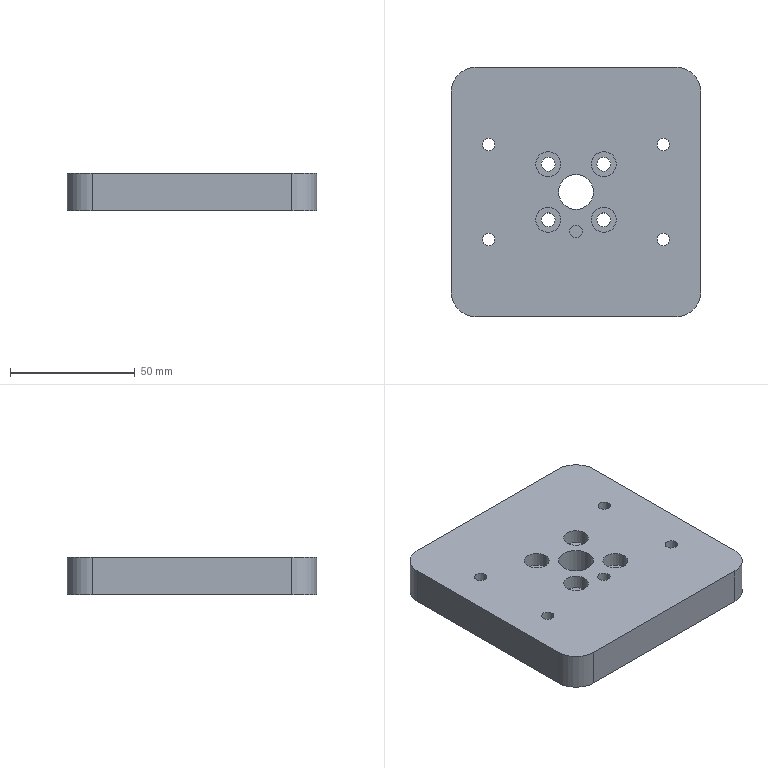Part | NX | 1 solid | 31 faces | box 100 x 100 x 15 mm | volume 134688 mm3 | cylinder 19 | plane 12 | commonest cylinder face diameters 5 x5 5.5 x4 10 x4 20 x4 14 x1 60 x1
STEP:
#1=CARTESIAN_POINT('',(186.874,129.988,-5.7));
#2=VERTEX_POINT('',#1);
#3=CARTESIAN_POINT('',(184.124,129.988,-5.7));
#4=DIRECTION('',(0.,0.,1.));
#5=DIRECTION('',(1.,0.,0.));
#6=AXIS2_PLACEMENT_3D('',#3,#4,#5);
#7=CIRCLE('',#6,2.75);
#8=EDGE_CURVE('',#2,#2,#7,.F.);
#9=ORIENTED_EDGE('',*,*,#8,.F.);
#10=EDGE_LOOP('',(#9));
#11=FACE_BOUND('',#10,.T.);
#12=CARTESIAN_POINT('',(181.374,129.988,-12.));
#13=VERTEX_POINT('',#12);
#14=CARTESIAN_POINT('',(184.124,129.988,-12.));
#15=DIRECTION('',(0.,0.,-1.));
#16=DIRECTION('',(-1.,0.,0.));
#17=AXIS2_PLACEMENT_3D('',#14,#15,#16);
#18=CIRCLE('',#17,2.75);
#19=EDGE_CURVE('',#13,#13,#18,.F.);
#20=ORIENTED_EDGE('',*,*,#19,.F.);
#21=EDGE_LOOP('',(#20));
#22=FACE_BOUND('',#21,.T.);
#23=CARTESIAN_POINT('',(184.124,129.988,-15.));
#24=DIRECTION('',(0.,0.,1.));
#25=DIRECTION('',(1.,0.,0.));
#26=AXIS2_PLACEMENT_3D('',#23,#24,#25);
#27=CYLINDRICAL_SURFACE('',#26,2.75);
#28=ADVANCED_FACE('',(#11,#22),#27,.F.);
#29=CARTESIAN_POINT('',(186.874,107.714,-5.7));
#30=VERTEX_POINT('',#29);
#31=CARTESIAN_POINT('',(184.124,107.714,-5.7));
#32=DIRECTION('',(0.,0.,1.));
#33=DIRECTION('',(1.,0.,0.));
#34=AXIS2_PLACEMENT_3D('',#31,#32,#33);
#35=CIRCLE('',#34,2.75);
#36=EDGE_CURVE('',#30,#30,#35,.F.);
#37=ORIENTED_EDGE('',*,*,#36,.F.);
#38=EDGE_LOOP('',(#37));
#39=FACE_BOUND('',#38,.T.);
#40=CARTESIAN_POINT('',(181.374,107.714,-12.));
#41=VERTEX_POINT('',#40);
#42=CARTESIAN_POINT('',(184.124,107.714,-12.));
#43=DIRECTION('',(0.,0.,-1.));
#44=DIRECTION('',(-1.,0.,0.));
#45=AXIS2_PLACEMENT_3D('',#42,#43,#44);
#46=CIRCLE('',#45,2.75);
#47=EDGE_CURVE('',#41,#41,#46,.F.);
#48=ORIENTED_EDGE('',*,*,#47,.F.);
#49=EDGE_LOOP('',(#48));
#50=FACE_BOUND('',#49,.T.);
#51=CARTESIAN_POINT('',(184.124,107.714,-15.));
#52=DIRECTION('',(0.,0.,1.));
#53=DIRECTION('',(1.,0.,0.));
#54=AXIS2_PLACEMENT_3D('',#51,#52,#53);
#55=CYLINDRICAL_SURFACE('',#54,2.75);
#56=ADVANCED_FACE('',(#39,#50),#55,.F.);
#57=CARTESIAN_POINT('',(164.6,129.988,-5.7));
#58=VERTEX_POINT('',#57);
#59=CARTESIAN_POINT('',(161.85,129.988,-5.7));
#60=DIRECTION('',(0.,0.,1.));
#61=DIRECTION('',(1.,0.,0.));
#62=AXIS2_PLACEMENT_3D('',#59,#60,#61);
#63=CIRCLE('',#62,2.75);
#64=EDGE_CURVE('',#58,#58,#63,.F.);
#65=ORIENTED_EDGE('',*,*,#64,.F.);
#66=EDGE_LOOP('',(#65));
#67=FACE_BOUND('',#66,.T.);
#68=CARTESIAN_POINT('',(159.1,129.988,-12.));
#69=VERTEX_POINT('',#68);
#70=CARTESIAN_POINT('',(161.85,129.988,-12.));
#71=DIRECTION('',(0.,0.,-1.));
#72=DIRECTION('',(-1.,0.,0.));
#73=AXIS2_PLACEMENT_3D('',#70,#71,#72);
#74=CIRCLE('',#73,2.75);
#75=EDGE_CURVE('',#69,#69,#74,.F.);
#76=ORIENTED_EDGE('',*,*,#75,.F.);
#77=EDGE_LOOP('',(#76));
#78=FACE_BOUND('',#77,.T.);
#79=CARTESIAN_POINT('',(161.85,129.988,-15.));
#80=DIRECTION('',(0.,0.,1.));
#81=DIRECTION('',(1.,0.,0.));
#82=AXIS2_PLACEMENT_3D('',#79,#80,#81);
#83=CYLINDRICAL_SURFACE('',#82,2.75);
#84=ADVANCED_FACE('',(#67,#78),#83,.F.);
#85=CARTESIAN_POINT('',(164.6,107.714,-5.7));
#86=VERTEX_POINT('',#85);
#87=CARTESIAN_POINT('',(161.85,107.714,-5.7));
#88=DIRECTION('',(0.,0.,1.));
#89=DIRECTION('',(1.,0.,0.));
#90=AXIS2_PLACEMENT_3D('',#87,#88,#89);
#91=CIRCLE('',#90,2.75);
#92=EDGE_CURVE('',#86,#86,#91,.F.);
#93=ORIENTED_EDGE('',*,*,#92,.F.);
#94=EDGE_LOOP('',(#93));
#95=FACE_BOUND('',#94,.T.);
#96=CARTESIAN_POINT('',(159.1,107.714,-12.));
#97=VERTEX_POINT('',#96);
#98=CARTESIAN_POINT('',(161.85,107.714,-12.));
#99=DIRECTION('',(0.,0.,-1.));
#100=DIRECTION('',(-1.,0.,0.));
#101=AXIS2_PLACEMENT_3D('',#98,#99,#100);
#102=CIRCLE('',#101,2.75);
#103=EDGE_CURVE('',#97,#97,#102,.F.);
#104=ORIENTED_EDGE('',*,*,#103,.F.);
#105=EDGE_LOOP('',(#104));
#106=FACE_BOUND('',#105,.T.);
#107=CARTESIAN_POINT('',(161.85,107.714,-15.));
#108=DIRECTION('',(0.,0.,1.));
#109=DIRECTION('',(1.,0.,0.));
#110=AXIS2_PLACEMENT_3D('',#107,#108,#109);
#111=CYLINDRICAL_SURFACE('',#110,2.75);
#112=ADVANCED_FACE('',(#95,#106),#111,.F.);
#113=CARTESIAN_POINT('',(179.987,118.851,0.));
#114=VERTEX_POINT('',#113);
#115=CARTESIAN_POINT('',(172.987,118.851,0.));
#116=DIRECTION('',(0.,0.,1.));
#117=DIRECTION('',(1.,0.,0.));
#118=AXIS2_PLACEMENT_3D('',#115,#116,#117);
#119=CIRCLE('',#118,7.);
#120=EDGE_CURVE('',#114,#114,#119,.T.);
#121=ORIENTED_EDGE('',*,*,#120,.T.);
#122=EDGE_LOOP('',(#121));
#123=FACE_BOUND('',#122,.T.);
#124=CARTESIAN_POINT('',(165.987,118.851,-12.));
#125=VERTEX_POINT('',#124);
#126=CARTESIAN_POINT('',(172.987,118.851,-12.));
#127=DIRECTION('',(0.,0.,-1.));
#128=DIRECTION('',(-1.,0.,0.));
#129=AXIS2_PLACEMENT_3D('',#126,#127,#128);
#130=CIRCLE('',#129,7.);
#131=EDGE_CURVE('',#125,#125,#130,.F.);
#132=ORIENTED_EDGE('',*,*,#131,.F.);
#133=EDGE_LOOP('',(#132));
#134=FACE_BOUND('',#133,.T.);
#135=CARTESIAN_POINT('',(172.987,118.851,-15.));
#136=DIRECTION('',(0.,0.,1.));
#137=DIRECTION('',(1.,0.,0.));
#138=AXIS2_PLACEMENT_3D('',#135,#136,#137);
#139=CYLINDRICAL_SURFACE('',#138,7.);
#140=ADVANCED_FACE('',(#123,#134),#139,.F.);
#141=CARTESIAN_POINT('',(122.987,158.851,0.));
#142=VERTEX_POINT('',#141);
#143=CARTESIAN_POINT('',(122.987,78.851,0.));
#144=VERTEX_POINT('',#143);
#145=CARTESIAN_POINT('',(122.987,158.851,0.));
#146=DIRECTION('',(0.,-1.,0.));
#147=VECTOR('',#146,1000.);
#148=LINE('',#145,#147);
#149=EDGE_CURVE('',#142,#144,#148,.T.);
#150=ORIENTED_EDGE('',*,*,#149,.F.);
#151=CARTESIAN_POINT('',(122.987,158.851,-15.));
#152=VERTEX_POINT('',#151);
#153=CARTESIAN_POINT('',(122.987,158.851,-15.));
#154=DIRECTION('',(0.,0.,1.));
#155=VECTOR('',#154,1000.);
#156=LINE('',#153,#155);
#157=EDGE_CURVE('',#152,#142,#156,.T.);
#158=ORIENTED_EDGE('',*,*,#157,.F.);
#159=CARTESIAN_POINT('',(122.987,78.851,-15.));
#160=VERTEX_POINT('',#159);
#161=CARTESIAN_POINT('',(122.987,158.851,-15.));
#162=DIRECTION('',(0.,-1.,0.));
#163=VECTOR('',#162,1000.);
#164=LINE('',#161,#163);
#165=EDGE_CURVE('',#152,#160,#164,.T.);
#166=ORIENTED_EDGE('',*,*,#165,.T.);
#167=CARTESIAN_POINT('',(122.987,78.851,-15.));
#168=DIRECTION('',(0.,0.,1.));
#169=VECTOR('',#168,1000.);
#170=LINE('',#167,#169);
#171=EDGE_CURVE('',#160,#144,#170,.T.);
#172=ORIENTED_EDGE('',*,*,#171,.T.);
#173=EDGE_LOOP('',(#150,#158,#166,#172));
#174=FACE_BOUND('',#173,.T.);
#175=CARTESIAN_POINT('',(122.987,158.851,-15.));
#176=DIRECTION('',(-1.,0.,0.));
#177=DIRECTION('',(0.,0.,1.));
#178=AXIS2_PLACEMENT_3D('',#175,#176,#177);
#179=PLANE('',#178);
#180=ADVANCED_FACE('',(#174),#179,.T.);
#181=CARTESIAN_POINT('',(132.987,68.851,0.));
#182=VERTEX_POINT('',#181);
#183=CARTESIAN_POINT('',(132.987,78.851,0.));
#184=DIRECTION('',(0.,0.,1.));
#185=DIRECTION('',(1.,0.,0.));
#186=AXIS2_PLACEMENT_3D('',#183,#184,#185);
#187=CIRCLE('',#186,10.);
#188=EDGE_CURVE('',#144,#182,#187,.T.);
#189=ORIENTED_EDGE('',*,*,#188,.F.);
#190=ORIENTED_EDGE('',*,*,#171,.F.);
#191=CARTESIAN_POINT('',(132.987,68.851,-15.));
#192=VERTEX_POINT('',#191);
#193=CARTESIAN_POINT('',(132.987,78.851,-15.));
#194=DIRECTION('',(0.,0.,1.));
#195=DIRECTION('',(1.,0.,0.));
#196=AXIS2_PLACEMENT_3D('',#193,#194,#195);
#197=CIRCLE('',#196,10.);
#198=EDGE_CURVE('',#160,#192,#197,.T.);
#199=ORIENTED_EDGE('',*,*,#198,.T.);
#200=CARTESIAN_POINT('',(132.987,68.851,-15.));
#201=DIRECTION('',(0.,0.,1.));
#202=VECTOR('',#201,1000.);
#203=LINE('',#200,#202);
#204=EDGE_CURVE('',#192,#182,#203,.T.);
#205=ORIENTED_EDGE('',*,*,#204,.T.);
#206=EDGE_LOOP('',(#189,#190,#199,#205));
#207=FACE_BOUND('',#206,.T.);
#208=CARTESIAN_POINT('',(132.987,78.851,-15.));
#209=DIRECTION('',(0.,0.,1.));
#210=DIRECTION('',(1.,0.,0.));
#211=AXIS2_PLACEMENT_3D('',#208,#209,#210);
#212=CYLINDRICAL_SURFACE('',#211,10.);
#213=ADVANCED_FACE('',(#207),#212,.T.);
#214=CARTESIAN_POINT('',(212.987,68.851,0.));
#215=VERTEX_POINT('',#214);
#216=CARTESIAN_POINT('',(132.987,68.851,0.));
#217=DIRECTION('',(1.,0.,0.));
#218=VECTOR('',#217,1000.);
#219=LINE('',#216,#218);
#220=EDGE_CURVE('',#182,#215,#219,.T.);
#221=ORIENTED_EDGE('',*,*,#220,.F.);
#222=ORIENTED_EDGE('',*,*,#204,.F.);
#223=CARTESIAN_POINT('',(212.987,68.851,-15.));
#224=VERTEX_POINT('',#223);
#225=CARTESIAN_POINT('',(132.987,68.851,-15.));
#226=DIRECTION('',(1.,0.,0.));
#227=VECTOR('',#226,1000.);
#228=LINE('',#225,#227);
#229=EDGE_CURVE('',#192,#224,#228,.T.);
#230=ORIENTED_EDGE('',*,*,#229,.T.);
#231=CARTESIAN_POINT('',(212.987,68.851,-15.));
#232=DIRECTION('',(0.,0.,1.));
#233=VECTOR('',#232,1000.);
#234=LINE('',#231,#233);
#235=EDGE_CURVE('',#224,#215,#234,.T.);
#236=ORIENTED_EDGE('',*,*,#235,.T.);
#237=EDGE_LOOP('',(#221,#222,#230,#236));
#238=FACE_BOUND('',#237,.T.);
#239=CARTESIAN_POINT('',(132.987,68.851,-15.));
#240=DIRECTION('',(0.,-1.,0.));
#241=DIRECTION('',(0.,0.,-1.));
#242=AXIS2_PLACEMENT_3D('',#239,#240,#241);
#243=PLANE('',#242);
#244=ADVANCED_FACE('',(#238),#243,.T.);
#245=CARTESIAN_POINT('',(222.987,78.851,0.));
#246=VERTEX_POINT('',#245);
#247=CARTESIAN_POINT('',(212.987,78.851,0.));
#248=DIRECTION('',(0.,0.,1.));
#249=DIRECTION('',(1.,0.,0.));
#250=AXIS2_PLACEMENT_3D('',#247,#248,#249);
#251=CIRCLE('',#250,10.);
#252=EDGE_CURVE('',#215,#246,#251,.T.);
#253=ORIENTED_EDGE('',*,*,#252,.F.);
#254=ORIENTED_EDGE('',*,*,#235,.F.);
#255=CARTESIAN_POINT('',(222.987,78.851,-15.));
#256=VERTEX_POINT('',#255);
#257=CARTESIAN_POINT('',(212.987,78.851,-15.));
#258=DIRECTION('',(0.,0.,1.));
#259=DIRECTION('',(1.,0.,0.));
#260=AXIS2_PLACEMENT_3D('',#257,#258,#259);
#261=CIRCLE('',#260,10.);
#262=EDGE_CURVE('',#224,#256,#261,.T.);
#263=ORIENTED_EDGE('',*,*,#262,.T.);
#264=CARTESIAN_POINT('',(222.987,78.851,-15.));
#265=DIRECTION('',(0.,0.,1.));
#266=VECTOR('',#265,1000.);
#267=LINE('',#264,#266);
#268=EDGE_CURVE('',#256,#246,#267,.T.);
#269=ORIENTED_EDGE('',*,*,#268,.T.);
#270=EDGE_LOOP('',(#253,#254,#263,#269));
#271=FACE_BOUND('',#270,.T.);
#272=CARTESIAN_POINT('',(212.987,78.851,-15.));
#273=DIRECTION('',(0.,0.,1.));
#274=DIRECTION('',(1.,0.,0.));
#275=AXIS2_PLACEMENT_3D('',#272,#273,#274);
#276=CYLINDRICAL_SURFACE('',#275,10.);
#277=ADVANCED_FACE('',(#271),#276,.T.);
#278=CARTESIAN_POINT('',(222.987,158.851,0.));
#279=VERTEX_POINT('',#278);
#280=CARTESIAN_POINT('',(222.987,78.851,0.));
#281=DIRECTION('',(0.,1.,0.));
#282=VECTOR('',#281,1000.);
#283=LINE('',#280,#282);
#284=EDGE_CURVE('',#246,#279,#283,.T.);
#285=ORIENTED_EDGE('',*,*,#284,.F.);
#286=ORIENTED_EDGE('',*,*,#268,.F.);
#287=CARTESIAN_POINT('',(222.987,158.851,-15.));
#288=VERTEX_POINT('',#287);
#289=CARTESIAN_POINT('',(222.987,78.851,-15.));
#290=DIRECTION('',(0.,1.,0.));
#291=VECTOR('',#290,1000.);
#292=LINE('',#289,#291);
#293=EDGE_CURVE('',#256,#288,#292,.T.);
#294=ORIENTED_EDGE('',*,*,#293,.T.);
#295=CARTESIAN_POINT('',(222.987,158.851,-15.));
#296=DIRECTION('',(0.,0.,1.));
#297=VECTOR('',#296,1000.);
#298=LINE('',#295,#297);
#299=EDGE_CURVE('',#288,#279,#298,.T.);
#300=ORIENTED_EDGE('',*,*,#299,.T.);
#301=EDGE_LOOP('',(#285,#286,#294,#300));
#302=FACE_BOUND('',#301,.T.);
#303=CARTESIAN_POINT('',(222.987,78.851,-15.));
#304=DIRECTION('',(1.,0.,0.));
#305=DIRECTION('',(0.,0.,-1.));
#306=AXIS2_PLACEMENT_3D('',#303,#304,#305);
#307=PLANE('',#306);
#308=ADVANCED_FACE('',(#302),#307,.T.);
#309=CARTESIAN_POINT('',(212.987,168.851,0.));
#310=VERTEX_POINT('',#309);
#311=CARTESIAN_POINT('',(212.987,158.851,0.));
#312=DIRECTION('',(0.,0.,1.));
#313=DIRECTION('',(1.,0.,0.));
#314=AXIS2_PLACEMENT_3D('',#311,#312,#313);
#315=CIRCLE('',#314,10.);
#316=EDGE_CURVE('',#279,#310,#315,.T.);
#317=ORIENTED_EDGE('',*,*,#316,.F.);
#318=ORIENTED_EDGE('',*,*,#299,.F.);
#319=CARTESIAN_POINT('',(212.987,168.851,-15.));
#320=VERTEX_POINT('',#319);
#321=CARTESIAN_POINT('',(212.987,158.851,-15.));
#322=DIRECTION('',(0.,0.,1.));
#323=DIRECTION('',(1.,0.,0.));
#324=AXIS2_PLACEMENT_3D('',#321,#322,#323);
#325=CIRCLE('',#324,10.);
#326=EDGE_CURVE('',#288,#320,#325,.T.);
#327=ORIENTED_EDGE('',*,*,#326,.T.);
#328=CARTESIAN_POINT('',(212.987,168.851,-15.));
#329=DIRECTION('',(0.,0.,1.));
#330=VECTOR('',#329,1000.);
#331=LINE('',#328,#330);
#332=EDGE_CURVE('',#320,#310,#331,.T.);
#333=ORIENTED_EDGE('',*,*,#332,.T.);
#334=EDGE_LOOP('',(#317,#318,#327,#333));
#335=FACE_BOUND('',#334,.T.);
#336=CARTESIAN_POINT('',(212.987,158.851,-15.));
#337=DIRECTION('',(0.,0.,1.));
#338=DIRECTION('',(1.,0.,0.));
#339=AXIS2_PLACEMENT_3D('',#336,#337,#338);
#340=CYLINDRICAL_SURFACE('',#339,10.);
#341=ADVANCED_FACE('',(#335),#340,.T.);
#342=CARTESIAN_POINT('',(132.987,168.851,0.));
#343=VERTEX_POINT('',#342);
#344=CARTESIAN_POINT('',(212.987,168.851,0.));
#345=DIRECTION('',(-1.,0.,0.));
#346=VECTOR('',#345,1000.);
#347=LINE('',#344,#346);
#348=EDGE_CURVE('',#310,#343,#347,.T.);
#349=ORIENTED_EDGE('',*,*,#348,.F.);
#350=ORIENTED_EDGE('',*,*,#332,.F.);
#351=CARTESIAN_POINT('',(132.987,168.851,-15.));
#352=VERTEX_POINT('',#351);
#353=CARTESIAN_POINT('',(212.987,168.851,-15.));
#354=DIRECTION('',(-1.,0.,0.));
#355=VECTOR('',#354,1000.);
#356=LINE('',#353,#355);
#357=EDGE_CURVE('',#320,#352,#356,.T.);
#358=ORIENTED_EDGE('',*,*,#357,.T.);
#359=CARTESIAN_POINT('',(132.987,168.851,-15.));
#360=DIRECTION('',(0.,0.,1.));
#361=VECTOR('',#360,1000.);
#362=LINE('',#359,#361);
#363=EDGE_CURVE('',#352,#343,#362,.T.);
#364=ORIENTED_EDGE('',*,*,#363,.T.);
#365=EDGE_LOOP('',(#349,#350,#358,#364));
#366=FACE_BOUND('',#365,.T.);
#367=CARTESIAN_POINT('',(212.987,168.851,-15.));
#368=DIRECTION('',(0.,1.,0.));
#369=DIRECTION('',(0.,0.,1.));
#370=AXIS2_PLACEMENT_3D('',#367,#368,#369);
#371=PLANE('',#370);
#372=ADVANCED_FACE('',(#366),#371,.T.);
#373=CARTESIAN_POINT('',(210.487,99.851,-15.));
#374=VERTEX_POINT('',#373);
#375=CARTESIAN_POINT('',(207.987,99.851,-15.));
#376=DIRECTION('',(0.,0.,1.));
#377=DIRECTION('',(1.,0.,0.));
#378=AXIS2_PLACEMENT_3D('',#375,#376,#377);
#379=CIRCLE('',#378,2.5);
#380=EDGE_CURVE('',#374,#374,#379,.T.);
#381=ORIENTED_EDGE('',*,*,#380,.F.);
#382=EDGE_LOOP('',(#381));
#383=FACE_BOUND('',#382,.T.);
#384=CARTESIAN_POINT('',(210.487,99.851,0.));
#385=VERTEX_POINT('',#384);
#386=CARTESIAN_POINT('',(207.987,99.851,0.));
#387=DIRECTION('',(0.,0.,1.));
#388=DIRECTION('',(1.,0.,0.));
#389=AXIS2_PLACEMENT_3D('',#386,#387,#388);
#390=CIRCLE('',#389,2.5);
#391=EDGE_CURVE('',#385,#385,#390,.T.);
#392=ORIENTED_EDGE('',*,*,#391,.T.);
#393=EDGE_LOOP('',(#392));
#394=FACE_BOUND('',#393,.T.);
#395=CARTESIAN_POINT('',(207.987,99.851,-15.));
#396=DIRECTION('',(0.,0.,1.));
#397=DIRECTION('',(1.,0.,0.));
#398=AXIS2_PLACEMENT_3D('',#395,#396,#397);
#399=CYLINDRICAL_SURFACE('',#398,2.5);
#400=ADVANCED_FACE('',(#383,#394),#399,.F.);
#401=CARTESIAN_POINT('',(140.487,137.851,-15.));
#402=VERTEX_POINT('',#401);
#403=CARTESIAN_POINT('',(137.987,137.851,-15.));
#404=DIRECTION('',(0.,0.,1.));
#405=DIRECTION('',(1.,0.,0.));
#406=AXIS2_PLACEMENT_3D('',#403,#404,#405);
#407=CIRCLE('',#406,2.5);
#408=EDGE_CURVE('',#402,#402,#407,.T.);
#409=ORIENTED_EDGE('',*,*,#408,.F.);
#410=EDGE_LOOP('',(#409));
#411=FACE_BOUND('',#410,.T.);
#412=CARTESIAN_POINT('',(140.487,137.851,0.));
#413=VERTEX_POINT('',#412);
#414=CARTESIAN_POINT('',(137.987,137.851,0.));
#415=DIRECTION('',(0.,0.,1.));
#416=DIRECTION('',(1.,0.,0.));
#417=AXIS2_PLACEMENT_3D('',#414,#415,#416);
#418=CIRCLE('',#417,2.5);
#419=EDGE_CURVE('',#413,#413,#418,.T.);
#420=ORIENTED_EDGE('',*,*,#419,.T.);
#421=EDGE_LOOP('',(#420));
#422=FACE_BOUND('',#421,.T.);
#423=CARTESIAN_POINT('',(137.987,137.851,-15.));
#424=DIRECTION('',(0.,0.,1.));
#425=DIRECTION('',(1.,0.,0.));
#426=AXIS2_PLACEMENT_3D('',#423,#424,#425);
#427=CYLINDRICAL_SURFACE('',#426,2.5);
#428=ADVANCED_FACE('',(#411,#422),#427,.F.);
#429=CARTESIAN_POINT('',(140.487,99.851,-15.));
#430=VERTEX_POINT('',#429);
#431=CARTESIAN_POINT('',(137.987,99.851,-15.));
#432=DIRECTION('',(0.,0.,1.));
#433=DIRECTION('',(1.,0.,0.));
#434=AXIS2_PLACEMENT_3D('',#431,#432,#433);
#435=CIRCLE('',#434,2.5);
#436=EDGE_CURVE('',#430,#430,#435,.T.);
#437=ORIENTED_EDGE('',*,*,#436,.F.);
#438=EDGE_LOOP('',(#437));
#439=FACE_BOUND('',#438,.T.);
#440=CARTESIAN_POINT('',(140.487,99.851,0.));
#441=VERTEX_POINT('',#440);
#442=CARTESIAN_POINT('',(137.987,99.851,0.));
#443=DIRECTION('',(0.,0.,1.));
#444=DIRECTION('',(1.,0.,0.));
#445=AXIS2_PLACEMENT_3D('',#442,#443,#444);
#446=CIRCLE('',#445,2.5);
#447=EDGE_CURVE('',#441,#441,#446,.T.);
#448=ORIENTED_EDGE('',*,*,#447,.T.);
#449=EDGE_LOOP('',(#448));
#450=FACE_BOUND('',#449,.T.);
#451=CARTESIAN_POINT('',(137.987,99.851,-15.));
#452=DIRECTION('',(0.,0.,1.));
#453=DIRECTION('',(1.,0.,0.));
#454=AXIS2_PLACEMENT_3D('',#451,#452,#453);
#455=CYLINDRICAL_SURFACE('',#454,2.5);
#456=ADVANCED_FACE('',(#439,#450),#455,.F.);
#457=CARTESIAN_POINT('',(132.987,158.851,0.));
#458=DIRECTION('',(0.,0.,1.));
#459=DIRECTION('',(1.,0.,0.));
#460=AXIS2_PLACEMENT_3D('',#457,#458,#459);
#461=CIRCLE('',#460,10.);
#462=EDGE_CURVE('',#343,#142,#461,.T.);
#463=ORIENTED_EDGE('',*,*,#462,.F.);
#464=ORIENTED_EDGE('',*,*,#363,.F.);
#465=CARTESIAN_POINT('',(132.987,158.851,-15.));
#466=DIRECTION('',(0.,0.,1.));
#467=DIRECTION('',(1.,0.,0.));
#468=AXIS2_PLACEMENT_3D('',#465,#466,#467);
#469=CIRCLE('',#468,10.);
#470=EDGE_CURVE('',#352,#152,#469,.T.);
#471=ORIENTED_EDGE('',*,*,#470,.T.);
#472=ORIENTED_EDGE('',*,*,#157,.T.);
#473=EDGE_LOOP('',(#463,#464,#471,#472));
#474=FACE_BOUND('',#473,.T.);
#475=CARTESIAN_POINT('',(132.987,158.851,-15.));
#476=DIRECTION('',(0.,0.,1.));
#477=DIRECTION('',(1.,0.,0.));
#478=AXIS2_PLACEMENT_3D('',#475,#476,#477);
#479=CYLINDRICAL_SURFACE('',#478,10.);
#480=ADVANCED_FACE('',(#474),#479,.T.);
#481=CARTESIAN_POINT('',(210.487,137.851,-15.));
#482=VERTEX_POINT('',#481);
#483=CARTESIAN_POINT('',(207.987,137.851,-15.));
#484=DIRECTION('',(0.,0.,1.));
#485=DIRECTION('',(1.,0.,0.));
#486=AXIS2_PLACEMENT_3D('',#483,#484,#485);
#487=CIRCLE('',#486,2.5);
#488=EDGE_CURVE('',#482,#482,#487,.T.);
#489=ORIENTED_EDGE('',*,*,#488,.F.);
#490=EDGE_LOOP('',(#489));
#491=FACE_BOUND('',#490,.T.);
#492=CARTESIAN_POINT('',(210.487,137.851,0.));
#493=VERTEX_POINT('',#492);
#494=CARTESIAN_POINT('',(207.987,137.851,0.));
#495=DIRECTION('',(0.,0.,1.));
#496=DIRECTION('',(1.,0.,0.));
#497=AXIS2_PLACEMENT_3D('',#494,#495,#496);
#498=CIRCLE('',#497,2.5);
#499=EDGE_CURVE('',#493,#493,#498,.T.);
#500=ORIENTED_EDGE('',*,*,#499,.T.);
#501=EDGE_LOOP('',(#500));
#502=FACE_BOUND('',#501,.T.);
#503=CARTESIAN_POINT('',(207.987,137.851,-15.));
#504=DIRECTION('',(0.,0.,1.));
#505=DIRECTION('',(1.,0.,0.));
#506=AXIS2_PLACEMENT_3D('',#503,#504,#505);
#507=CYLINDRICAL_SURFACE('',#506,2.5);
#508=ADVANCED_FACE('',(#491,#502),#507,.F.);
#509=CARTESIAN_POINT('',(202.987,118.851,-15.));
#510=VERTEX_POINT('',#509);
#511=CARTESIAN_POINT('',(172.987,118.851,-15.));
#512=DIRECTION('',(0.,0.,-1.));
#513=DIRECTION('',(1.,0.,0.));
#514=AXIS2_PLACEMENT_3D('',#511,#512,#513);
#515=CIRCLE('',#514,30.);
#516=EDGE_CURVE('',#510,#510,#515,.T.);
#517=ORIENTED_EDGE('',*,*,#516,.F.);
#518=EDGE_LOOP('',(#517));
#519=FACE_BOUND('',#518,.T.);
#520=ORIENTED_EDGE('',*,*,#165,.F.);
#521=ORIENTED_EDGE('',*,*,#470,.F.);
#522=ORIENTED_EDGE('',*,*,#357,.F.);
#523=ORIENTED_EDGE('',*,*,#326,.F.);
#524=ORIENTED_EDGE('',*,*,#293,.F.);
#525=ORIENTED_EDGE('',*,*,#262,.F.);
#526=ORIENTED_EDGE('',*,*,#229,.F.);
#527=ORIENTED_EDGE('',*,*,#198,.F.);
#528=EDGE_LOOP('',(#520,#521,#522,#523,#524,#525,#526,#527));
#529=FACE_BOUND('',#528,.T.);
#530=ORIENTED_EDGE('',*,*,#436,.T.);
#531=EDGE_LOOP('',(#530));
#532=FACE_BOUND('',#531,.T.);
#533=ORIENTED_EDGE('',*,*,#408,.T.);
#534=EDGE_LOOP('',(#533));
#535=FACE_BOUND('',#534,.T.);
#536=ORIENTED_EDGE('',*,*,#380,.T.);
#537=EDGE_LOOP('',(#536));
#538=FACE_BOUND('',#537,.T.);
#539=ORIENTED_EDGE('',*,*,#488,.T.);
#540=EDGE_LOOP('',(#539));
#541=FACE_BOUND('',#540,.T.);
#542=CARTESIAN_POINT('',(132.987,78.851,-15.));
#543=DIRECTION('',(0.,0.,1.));
#544=DIRECTION('',(1.,0.,0.));
#545=AXIS2_PLACEMENT_3D('',#542,#543,#544);
#546=PLANE('',#545);
#547=ADVANCED_FACE('',(#519,#529,#532,#535,#538,#541),#546,.F.);
#548=CARTESIAN_POINT('',(189.124,107.714,0.));
#549=VERTEX_POINT('',#548);
#550=CARTESIAN_POINT('',(184.124,107.714,0.));
#551=DIRECTION('',(0.,0.,1.));
#552=DIRECTION('',(1.,0.,0.));
#553=AXIS2_PLACEMENT_3D('',#550,#551,#552);
#554=CIRCLE('',#553,5.);
#555=EDGE_CURVE('',#549,#549,#554,.T.);
#556=ORIENTED_EDGE('',*,*,#555,.F.);
#557=EDGE_LOOP('',(#556));
#558=FACE_BOUND('',#557,.T.);
#559=CARTESIAN_POINT('',(166.85,129.988,0.));
#560=VERTEX_POINT('',#559);
#561=CARTESIAN_POINT('',(161.85,129.988,0.));
#562=DIRECTION('',(0.,0.,1.));
#563=DIRECTION('',(1.,0.,0.));
#564=AXIS2_PLACEMENT_3D('',#561,#562,#563);
#565=CIRCLE('',#564,5.);
#566=EDGE_CURVE('',#560,#560,#565,.T.);
#567=ORIENTED_EDGE('',*,*,#566,.F.);
#568=EDGE_LOOP('',(#567));
#569=FACE_BOUND('',#568,.T.);
#570=CARTESIAN_POINT('',(166.85,107.714,0.));
#571=VERTEX_POINT('',#570);
#572=CARTESIAN_POINT('',(161.85,107.714,0.));
#573=DIRECTION('',(0.,0.,1.));
#574=DIRECTION('',(1.,0.,0.));
#575=AXIS2_PLACEMENT_3D('',#572,#573,#574);
#576=CIRCLE('',#575,5.);
#577=EDGE_CURVE('',#571,#571,#576,.T.);
#578=ORIENTED_EDGE('',*,*,#577,.F.);
#579=EDGE_LOOP('',(#578));
#580=FACE_BOUND('',#579,.T.);
#581=CARTESIAN_POINT('',(189.124,129.988,0.));
#582=VERTEX_POINT('',#581);
#583=CARTESIAN_POINT('',(184.124,129.988,0.));
#584=DIRECTION('',(0.,0.,1.));
#585=DIRECTION('',(1.,0.,0.));
#586=AXIS2_PLACEMENT_3D('',#583,#584,#585);
#587=CIRCLE('',#586,5.);
#588=EDGE_CURVE('',#582,#582,#587,.T.);
#589=ORIENTED_EDGE('',*,*,#588,.F.);
#590=EDGE_LOOP('',(#589));
#591=FACE_BOUND('',#590,.T.);
#592=CARTESIAN_POINT('',(175.487,103.101,0.));
#593=VERTEX_POINT('',#592);
#594=CARTESIAN_POINT('',(172.987,103.101,0.));
#595=DIRECTION('',(0.,0.,1.));
#596=DIRECTION('',(1.,0.,0.));
#597=AXIS2_PLACEMENT_3D('',#594,#595,#596);
#598=CIRCLE('',#597,2.5);
#599=EDGE_CURVE('',#593,#593,#598,.T.);
#600=ORIENTED_EDGE('',*,*,#599,.F.);
#601=EDGE_LOOP('',(#600));
#602=FACE_BOUND('',#601,.T.);
#603=ORIENTED_EDGE('',*,*,#149,.T.);
#604=ORIENTED_EDGE('',*,*,#188,.T.);
#605=ORIENTED_EDGE('',*,*,#220,.T.);
#606=ORIENTED_EDGE('',*,*,#252,.T.);
#607=ORIENTED_EDGE('',*,*,#284,.T.);
#608=ORIENTED_EDGE('',*,*,#316,.T.);
#609=ORIENTED_EDGE('',*,*,#348,.T.);
#610=ORIENTED_EDGE('',*,*,#462,.T.);
#611=EDGE_LOOP('',(#603,#604,#605,#606,#607,#608,#609,#610));
#612=FACE_BOUND('',#611,.T.);
#613=ORIENTED_EDGE('',*,*,#447,.F.);
#614=EDGE_LOOP('',(#613));
#615=FACE_BOUND('',#614,.T.);
#616=ORIENTED_EDGE('',*,*,#419,.F.);
#617=EDGE_LOOP('',(#616));
#618=FACE_BOUND('',#617,.T.);
#619=ORIENTED_EDGE('',*,*,#120,.F.);
#620=EDGE_LOOP('',(#619));
#621=FACE_BOUND('',#620,.T.);
#622=ORIENTED_EDGE('',*,*,#391,.F.);
#623=EDGE_LOOP('',(#622));
#624=FACE_BOUND('',#623,.T.);
#625=ORIENTED_EDGE('',*,*,#499,.F.);
#626=EDGE_LOOP('',(#625));
#627=FACE_BOUND('',#626,.T.);
#628=CARTESIAN_POINT('',(132.987,78.851,0.));
#629=DIRECTION('',(0.,0.,1.));
#630=DIRECTION('',(1.,0.,0.));
#631=AXIS2_PLACEMENT_3D('',#628,#629,#630);
#632=PLANE('',#631);
#633=ADVANCED_FACE('',(#558,#569,#580,#591,#602,#612,#615,#618,#621,#624,#627),#632,.T.);
#634=CARTESIAN_POINT('',(175.487,103.101,-6.5));
#635=VERTEX_POINT('',#634);
#636=CARTESIAN_POINT('',(172.987,103.101,-6.5));
#637=DIRECTION('',(0.,0.,1.));
#638=DIRECTION('',(1.,0.,0.));
#639=AXIS2_PLACEMENT_3D('',#636,#637,#638);
#640=CIRCLE('',#639,2.5);
#641=EDGE_CURVE('',#635,#635,#640,.F.);
#642=ORIENTED_EDGE('',*,*,#641,.T.);
#643=EDGE_LOOP('',(#642));
#644=FACE_BOUND('',#643,.T.);
#645=ORIENTED_EDGE('',*,*,#599,.T.);
#646=EDGE_LOOP('',(#645));
#647=FACE_BOUND('',#646,.T.);
#648=CARTESIAN_POINT('',(172.987,103.101,-6.5));
#649=DIRECTION('',(0.,0.,1.));
#650=DIRECTION('',(1.,0.,0.));
#651=AXIS2_PLACEMENT_3D('',#648,#649,#650);
#652=CYLINDRICAL_SURFACE('',#651,2.5);
#653=ADVANCED_FACE('',(#644,#647),#652,.F.);
#654=ORIENTED_EDGE('',*,*,#641,.F.);
#655=EDGE_LOOP('',(#654));
#656=FACE_BOUND('',#655,.T.);
#657=CARTESIAN_POINT('',(172.987,103.101,-6.5));
#658=DIRECTION('',(0.,0.,1.));
#659=DIRECTION('',(1.,0.,0.));
#660=AXIS2_PLACEMENT_3D('',#657,#658,#659);
#661=PLANE('',#660);
#662=ADVANCED_FACE('',(#656),#661,.T.);
#663=CARTESIAN_POINT('',(189.124,129.988,-5.7));
#664=VERTEX_POINT('',#663);
#665=CARTESIAN_POINT('',(184.124,129.988,-5.7));
#666=DIRECTION('',(0.,0.,1.));
#667=DIRECTION('',(1.,0.,0.));
#668=AXIS2_PLACEMENT_3D('',#665,#666,#667);
#669=CIRCLE('',#668,5.);
#670=EDGE_CURVE('',#664,#664,#669,.F.);
#671=ORIENTED_EDGE('',*,*,#670,.F.);
#672=EDGE_LOOP('',(#671));
#673=FACE_BOUND('',#672,.T.);
#674=ORIENTED_EDGE('',*,*,#8,.T.);
#675=EDGE_LOOP('',(#674));
#676=FACE_BOUND('',#675,.T.);
#677=CARTESIAN_POINT('',(184.124,129.988,-5.7));
#678=DIRECTION('',(0.,0.,1.));
#679=DIRECTION('',(1.,0.,0.));
#680=AXIS2_PLACEMENT_3D('',#677,#678,#679);
#681=PLANE('',#680);
#682=ADVANCED_FACE('',(#673,#676),#681,.T.);
#683=ORIENTED_EDGE('',*,*,#670,.T.);
#684=EDGE_LOOP('',(#683));
#685=FACE_BOUND('',#684,.T.);
#686=ORIENTED_EDGE('',*,*,#588,.T.);
#687=EDGE_LOOP('',(#686));
#688=FACE_BOUND('',#687,.T.);
#689=CARTESIAN_POINT('',(184.124,129.988,-5.7));
#690=DIRECTION('',(0.,0.,1.));
#691=DIRECTION('',(1.,0.,0.));
#692=AXIS2_PLACEMENT_3D('',#689,#690,#691);
#693=CYLINDRICAL_SURFACE('',#692,5.);
#694=ADVANCED_FACE('',(#685,#688),#693,.F.);
#695=CARTESIAN_POINT('',(166.85,107.714,-5.7));
#696=VERTEX_POINT('',#695);
#697=CARTESIAN_POINT('',(161.85,107.714,-5.7));
#698=DIRECTION('',(0.,0.,1.));
#699=DIRECTION('',(1.,0.,0.));
#700=AXIS2_PLACEMENT_3D('',#697,#698,#699);
#701=CIRCLE('',#700,5.);
#702=EDGE_CURVE('',#696,#696,#701,.F.);
#703=ORIENTED_EDGE('',*,*,#702,.F.);
#704=EDGE_LOOP('',(#703));
#705=FACE_BOUND('',#704,.T.);
#706=ORIENTED_EDGE('',*,*,#92,.T.);
#707=EDGE_LOOP('',(#706));
#708=FACE_BOUND('',#707,.T.);
#709=CARTESIAN_POINT('',(161.85,107.714,-5.7));
#710=DIRECTION('',(0.,0.,1.));
#711=DIRECTION('',(1.,0.,0.));
#712=AXIS2_PLACEMENT_3D('',#709,#710,#711);
#713=PLANE('',#712);
#714=ADVANCED_FACE('',(#705,#708),#713,.T.);
#715=ORIENTED_EDGE('',*,*,#702,.T.);
#716=EDGE_LOOP('',(#715));
#717=FACE_BOUND('',#716,.T.);
#718=ORIENTED_EDGE('',*,*,#577,.T.);
#719=EDGE_LOOP('',(#718));
#720=FACE_BOUND('',#719,.T.);
#721=CARTESIAN_POINT('',(161.85,107.714,-5.7));
#722=DIRECTION('',(0.,0.,1.));
#723=DIRECTION('',(1.,0.,0.));
#724=AXIS2_PLACEMENT_3D('',#721,#722,#723);
#725=CYLINDRICAL_SURFACE('',#724,5.);
#726=ADVANCED_FACE('',(#717,#720),#725,.F.);
#727=CARTESIAN_POINT('',(166.85,129.988,-5.7));
#728=VERTEX_POINT('',#727);
#729=CARTESIAN_POINT('',(161.85,129.988,-5.7));
#730=DIRECTION('',(0.,0.,1.));
#731=DIRECTION('',(1.,0.,0.));
#732=AXIS2_PLACEMENT_3D('',#729,#730,#731);
#733=CIRCLE('',#732,5.);
#734=EDGE_CURVE('',#728,#728,#733,.F.);
#735=ORIENTED_EDGE('',*,*,#734,.F.);
#736=EDGE_LOOP('',(#735));
#737=FACE_BOUND('',#736,.T.);
#738=ORIENTED_EDGE('',*,*,#64,.T.);
#739=EDGE_LOOP('',(#738));
#740=FACE_BOUND('',#739,.T.);
#741=CARTESIAN_POINT('',(161.85,129.988,-5.7));
#742=DIRECTION('',(0.,0.,1.));
#743=DIRECTION('',(1.,0.,0.));
#744=AXIS2_PLACEMENT_3D('',#741,#742,#743);
#745=PLANE('',#744);
#746=ADVANCED_FACE('',(#737,#740),#745,.T.);
#747=ORIENTED_EDGE('',*,*,#734,.T.);
#748=EDGE_LOOP('',(#747));
#749=FACE_BOUND('',#748,.T.);
#750=ORIENTED_EDGE('',*,*,#566,.T.);
#751=EDGE_LOOP('',(#750));
#752=FACE_BOUND('',#751,.T.);
#753=CARTESIAN_POINT('',(161.85,129.988,-5.7));
#754=DIRECTION('',(0.,0.,1.));
#755=DIRECTION('',(1.,0.,0.));
#756=AXIS2_PLACEMENT_3D('',#753,#754,#755);
#757=CYLINDRICAL_SURFACE('',#756,5.);
#758=ADVANCED_FACE('',(#749,#752),#757,.F.);
#759=CARTESIAN_POINT('',(189.124,107.714,-5.7));
#760=VERTEX_POINT('',#759);
#761=CARTESIAN_POINT('',(184.124,107.714,-5.7));
#762=DIRECTION('',(0.,0.,1.));
#763=DIRECTION('',(1.,0.,0.));
#764=AXIS2_PLACEMENT_3D('',#761,#762,#763);
#765=CIRCLE('',#764,5.);
#766=EDGE_CURVE('',#760,#760,#765,.F.);
#767=ORIENTED_EDGE('',*,*,#766,.F.);
#768=EDGE_LOOP('',(#767));
#769=FACE_BOUND('',#768,.T.);
#770=ORIENTED_EDGE('',*,*,#36,.T.);
#771=EDGE_LOOP('',(#770));
#772=FACE_BOUND('',#771,.T.);
#773=CARTESIAN_POINT('',(184.124,107.714,-5.7));
#774=DIRECTION('',(0.,0.,1.));
#775=DIRECTION('',(1.,0.,0.));
#776=AXIS2_PLACEMENT_3D('',#773,#774,#775);
#777=PLANE('',#776);
#778=ADVANCED_FACE('',(#769,#772),#777,.T.);
#779=ORIENTED_EDGE('',*,*,#766,.T.);
#780=EDGE_LOOP('',(#779));
#781=FACE_BOUND('',#780,.T.);
#782=ORIENTED_EDGE('',*,*,#555,.T.);
#783=EDGE_LOOP('',(#782));
#784=FACE_BOUND('',#783,.T.);
#785=CARTESIAN_POINT('',(184.124,107.714,-5.7));
#786=DIRECTION('',(0.,0.,1.));
#787=DIRECTION('',(1.,0.,0.));
#788=AXIS2_PLACEMENT_3D('',#785,#786,#787);
#789=CYLINDRICAL_SURFACE('',#788,5.);
#790=ADVANCED_FACE('',(#781,#784),#789,.F.);
#791=CARTESIAN_POINT('',(202.987,118.851,-12.));
#792=VERTEX_POINT('',#791);
#793=CARTESIAN_POINT('',(172.987,118.851,-12.));
#794=DIRECTION('',(0.,0.,-1.));
#795=DIRECTION('',(1.,0.,0.));
#796=AXIS2_PLACEMENT_3D('',#793,#794,#795);
#797=CIRCLE('',#796,30.);
#798=EDGE_CURVE('',#792,#792,#797,.F.);
#799=ORIENTED_EDGE('',*,*,#798,.F.);
#800=EDGE_LOOP('',(#799));
#801=FACE_BOUND('',#800,.T.);
#802=ORIENTED_EDGE('',*,*,#131,.T.);
#803=EDGE_LOOP('',(#802));
#804=FACE_BOUND('',#803,.T.);
#805=ORIENTED_EDGE('',*,*,#103,.T.);
#806=EDGE_LOOP('',(#805));
#807=FACE_BOUND('',#806,.T.);
#808=ORIENTED_EDGE('',*,*,#75,.T.);
#809=EDGE_LOOP('',(#808));
#810=FACE_BOUND('',#809,.T.);
#811=ORIENTED_EDGE('',*,*,#47,.T.);
#812=EDGE_LOOP('',(#811));
#813=FACE_BOUND('',#812,.T.);
#814=ORIENTED_EDGE('',*,*,#19,.T.);
#815=EDGE_LOOP('',(#814));
#816=FACE_BOUND('',#815,.T.);
#817=CARTESIAN_POINT('',(172.987,118.851,-12.));
#818=DIRECTION('',(0.,0.,-1.));
#819=DIRECTION('',(-1.,0.,0.));
#820=AXIS2_PLACEMENT_3D('',#817,#818,#819);
#821=PLANE('',#820);
#822=ADVANCED_FACE('',(#801,#804,#807,#810,#813,#816),#821,.T.);
#823=ORIENTED_EDGE('',*,*,#798,.T.);
#824=EDGE_LOOP('',(#823));
#825=FACE_BOUND('',#824,.T.);
#826=ORIENTED_EDGE('',*,*,#516,.T.);
#827=EDGE_LOOP('',(#826));
#828=FACE_BOUND('',#827,.T.);
#829=CARTESIAN_POINT('',(172.987,118.851,-12.));
#830=DIRECTION('',(0.,0.,-1.));
#831=DIRECTION('',(-1.,0.,0.));
#832=AXIS2_PLACEMENT_3D('',#829,#830,#831);
#833=CYLINDRICAL_SURFACE('',#832,30.);
#834=ADVANCED_FACE('',(#825,#828),#833,.F.);
#835=CLOSED_SHELL('',(#28,#56,#84,#112,#140,#180,#213,#244,#277,#308,#341,#372,#400,#428,#456,#480,#508,#547,#633,#653,#662,#682,#694,#714,#726,#746,#758,#778,#790,#822,#834));
#836=MANIFOLD_SOLID_BREP('',#835);
#837=(LENGTH_UNIT()NAMED_UNIT(*)SI_UNIT(.MILLI.,.METRE.));
#838=UNCERTAINTY_MEASURE_WITH_UNIT(LENGTH_MEASURE(0.00001),#837,'','');
#839=(NAMED_UNIT(*)PLANE_ANGLE_UNIT()SI_UNIT($,.RADIAN.));
#840=(NAMED_UNIT(*)SI_UNIT($,.STERADIAN.)SOLID_ANGLE_UNIT());
#841=(GEOMETRIC_REPRESENTATION_CONTEXT(3)GLOBAL_UNCERTAINTY_ASSIGNED_CONTEXT((#838))GLOBAL_UNIT_ASSIGNED_CONTEXT((#837,#839,#840))REPRESENTATION_CONTEXT('',''));
#842=ADVANCED_BREP_SHAPE_REPRESENTATION('',(#836),#841);